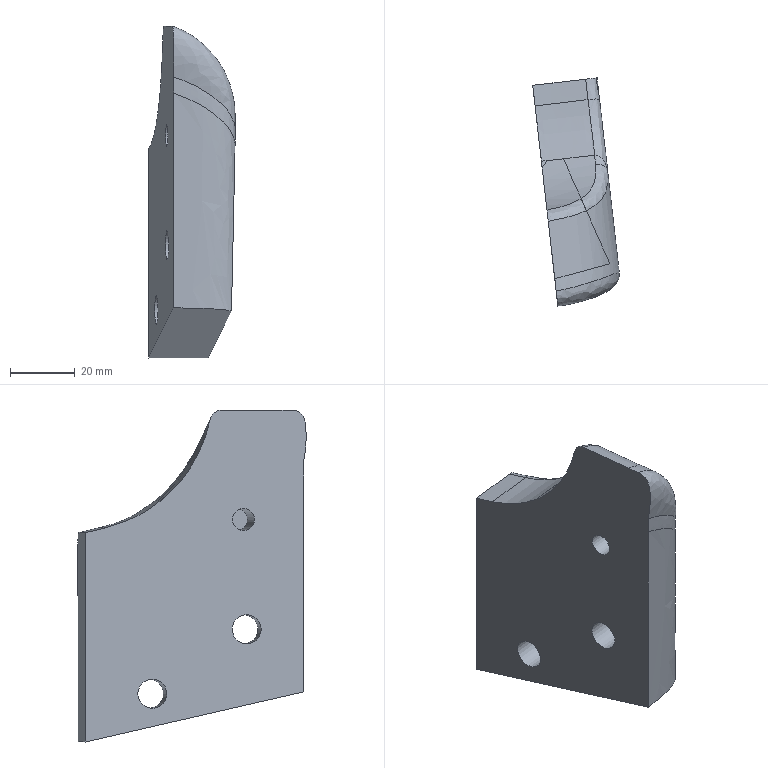Part | NX | features 23 2 | 1 solid | 42 faces | box 26.769 x 70.522 x 102.512 mm | volume 92072 mm3 | plane 17 | spline 15 | cylinder 10 | commonest cylinder face diameters 9 x2 14.5 x2 59 x2 87 x2 6.8 x1 7 x1